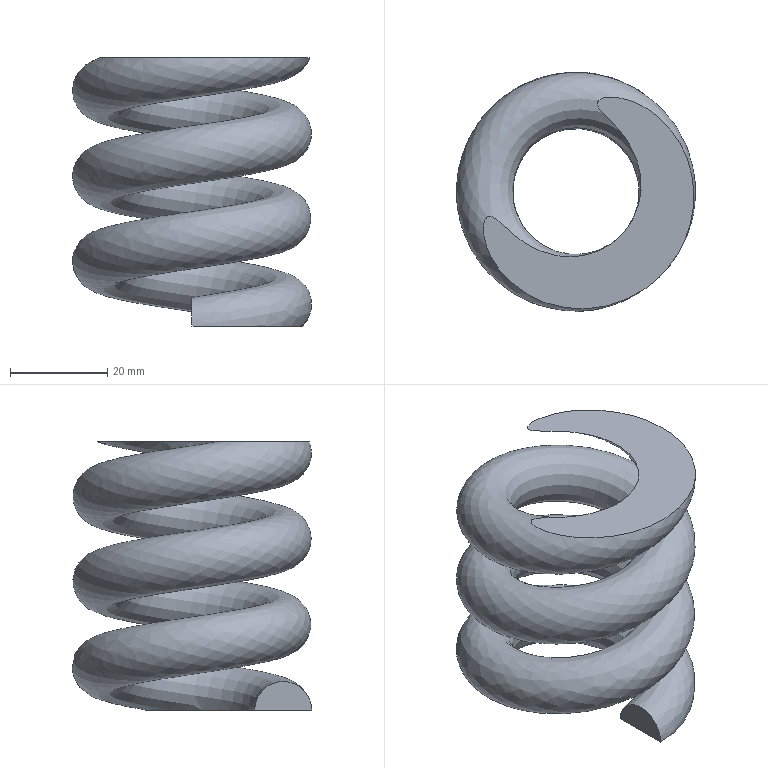Part | NX | features solid 2 | 1 solid | 4 faces | volume 38337 mm3 | plane 3 | spline 1
STEP:
#1=CARTESIAN_POINT('',(-1159.833,-619.642,-200.));
#2=VERTEX_POINT('',#1);
#3=CARTESIAN_POINT('',(-1159.833,-607.924,-200.));
#4=VERTEX_POINT('',#3);
#5=CARTESIAN_POINT('',(-1159.833,-613.783,-200.));
#6=DIRECTION('',(-1.,0.,0.));
#7=DIRECTION('',(0.,-1.,0.));
#8=AXIS2_PLACEMENT_3D('',#5,#6,#7);
#9=CIRCLE('',#8,5.859);
#10=EDGE_CURVE('',#2,#4,#9,.T.);
#11=ORIENTED_EDGE('',*,*,#10,.F.);
#12=CARTESIAN_POINT('',(-1159.833,-619.642,-200.));
#13=CARTESIAN_POINT('',(-1156.461,-619.642,-200.));
#14=CARTESIAN_POINT('',(-1151.454,-618.323,-200.));
#15=CARTESIAN_POINT('',(-1145.635,-614.786,-200.));
#16=CARTESIAN_POINT('',(-1141.941,-611.34,-200.));
#17=CARTESIAN_POINT('',(-1139.107,-607.051,-200.));
#18=CARTESIAN_POINT('',(-1137.419,-602.243,-200.));
#19=CARTESIAN_POINT('',(-1136.988,-598.021,-200.));
#20=CARTESIAN_POINT('',(-1137.288,-594.615,-200.));
#21=CARTESIAN_POINT('',(-1137.852,-592.138,-200.));
#22=CARTESIAN_POINT('',(-1138.795,-589.757,-200.));
#23=CARTESIAN_POINT('',(-1139.928,-587.928,-200.));
#24=CARTESIAN_POINT('',(-1141.068,-586.656,-200.));
#25=CARTESIAN_POINT('',(-1141.907,-585.972,-200.));
#26=CARTESIAN_POINT('',(-1142.679,-585.6,-200.));
#27=CARTESIAN_POINT('',(-1143.307,-585.474,-200.));
#28=CARTESIAN_POINT('',(-1143.919,-585.75,-200.));
#29=CARTESIAN_POINT('',(-1144.31,-586.53,-200.));
#30=CARTESIAN_POINT('',(-1144.432,-587.564,-200.));
#31=CARTESIAN_POINT('',(-1144.471,-588.818,-200.));
#32=CARTESIAN_POINT('',(-1144.484,-590.074,-200.));
#33=CARTESIAN_POINT('',(-1144.534,-591.747,-200.));
#34=CARTESIAN_POINT('',(-1144.72,-593.823,-200.));
#35=CARTESIAN_POINT('',(-1145.243,-596.307,-200.));
#36=CARTESIAN_POINT('',(-1146.08,-598.663,-200.));
#37=CARTESIAN_POINT('',(-1147.629,-601.639,-200.));
#38=CARTESIAN_POINT('',(-1150.333,-604.919,-200.));
#39=CARTESIAN_POINT('',(-1154.776,-607.425,-200.));
#40=CARTESIAN_POINT('',(-1158.142,-607.924,-200.));
#41=CARTESIAN_POINT('',(-1159.833,-607.924,-200.));
#42=B_SPLINE_CURVE_WITH_KNOTS('',3,(#12,#13,#14,#15,#16,#17,#18,#19,#20,#21,#22,#23,#24,#25,#26,#27,#28,#29,#30,#31,#32,#33,#34,#35,#36,#37,#38,#39,#40,#41),.UNSPECIFIED.,.F.,.F.,(4,1,1,1,1,1,1,1,1,1,1,1,1,1,1,1,1,1,1,1,1,1,1,1,1,1,1,4),(0.1116,0.1215,0.1265,0.1315,0.1365,0.1414,0.1464,0.1489,0.1514,0.1539,0.1564,0.1576,0.1589,0.1595,0.1601,0.1607,0.1614,0.1626,0.1639,0.1651,0.1664,0.1688,0.1713,0.1738,0.1763,0.1813,0.1863,0.1913),.UNSPECIFIED.);
#43=EDGE_CURVE('',#2,#4,#42,.T.);
#44=ORIENTED_EDGE('',*,*,#43,.T.);
#45=EDGE_LOOP('',(#11,#44));
#46=FACE_BOUND('',#45,.T.);
#47=CARTESIAN_POINT('',(-1176.496,-600.513,-145.));
#48=VERTEX_POINT('',#47);
#49=CARTESIAN_POINT('',(-1175.478,-601.297,-145.));
#50=CARTESIAN_POINT('',(-1176.301,-600.607,-145.));
#51=CARTESIAN_POINT('',(-1177.049,-600.187,-145.));
#52=CARTESIAN_POINT('',(-1177.712,-600.068,-145.));
#53=CARTESIAN_POINT('',(-1178.281,-600.447,-145.));
#54=CARTESIAN_POINT('',(-1178.67,-601.223,-145.));
#55=CARTESIAN_POINT('',(-1178.841,-602.282,-145.));
#56=CARTESIAN_POINT('',(-1178.808,-603.554,-145.));
#57=CARTESIAN_POINT('',(-1178.613,-604.806,-145.));
#58=CARTESIAN_POINT('',(-1178.177,-606.449,-145.));
#59=CARTESIAN_POINT('',(-1177.371,-608.377,-145.));
#60=CARTESIAN_POINT('',(-1176.039,-610.555,-145.));
#61=CARTESIAN_POINT('',(-1173.924,-613.138,-145.));
#62=CARTESIAN_POINT('',(-1170.662,-615.86,-145.));
#63=CARTESIAN_POINT('',(-1166.1,-618.088,-145.));
#64=CARTESIAN_POINT('',(-1161.184,-619.207,-145.));
#65=CARTESIAN_POINT('',(-1156.108,-619.164,-145.));
#66=CARTESIAN_POINT('',(-1149.523,-617.643,-145.));
#67=CARTESIAN_POINT('',(-1142.202,-613.198,-145.));
#68=CARTESIAN_POINT('',(-1137.495,-606.037,-145.));
#69=CARTESIAN_POINT('',(-1135.74,-599.515,-145.));
#70=CARTESIAN_POINT('',(-1135.504,-594.455,-145.));
#71=CARTESIAN_POINT('',(-1136.411,-589.51,-145.));
#72=CARTESIAN_POINT('',(-1138.445,-584.849,-145.));
#73=CARTESIAN_POINT('',(-1140.982,-581.484,-145.));
#74=CARTESIAN_POINT('',(-1143.469,-579.222,-145.));
#75=CARTESIAN_POINT('',(-1145.511,-577.795,-145.));
#76=CARTESIAN_POINT('',(-1147.787,-576.639,-145.));
#77=CARTESIAN_POINT('',(-1149.789,-575.994,-145.));
#78=CARTESIAN_POINT('',(-1151.467,-575.706,-145.));
#79=CARTESIAN_POINT('',(-1152.742,-575.639,-145.));
#80=CARTESIAN_POINT('',(-1153.795,-575.739,-145.));
#81=CARTESIAN_POINT('',(-1154.608,-575.989,-145.));
#82=CARTESIAN_POINT('',(-1155.181,-576.306,-145.));
#83=CARTESIAN_POINT('',(-1155.539,-576.891,-145.));
#84=CARTESIAN_POINT('',(-1155.386,-577.554,-145.));
#85=CARTESIAN_POINT('',(-1155.05,-578.094,-145.));
#86=CARTESIAN_POINT('',(-1154.509,-578.758,-145.));
#87=CARTESIAN_POINT('',(-1153.762,-579.518,-145.));
#88=CARTESIAN_POINT('',(-1152.548,-580.715,-145.));
#89=CARTESIAN_POINT('',(-1151.07,-582.261,-145.));
#90=CARTESIAN_POINT('',(-1149.001,-584.919,-145.));
#91=CARTESIAN_POINT('',(-1147.037,-588.717,-145.));
#92=CARTESIAN_POINT('',(-1146.153,-593.824,-145.));
#93=CARTESIAN_POINT('',(-1147.052,-598.911,-145.));
#94=CARTESIAN_POINT('',(-1149.587,-603.437,-145.));
#95=CARTESIAN_POINT('',(-1153.569,-606.748,-145.));
#96=CARTESIAN_POINT('',(-1158.449,-608.509,-145.));
#97=CARTESIAN_POINT('',(-1162.765,-608.529,-145.));
#98=CARTESIAN_POINT('',(-1166.065,-607.719,-145.));
#99=CARTESIAN_POINT('',(-1168.45,-606.738,-145.));
#100=CARTESIAN_POINT('',(-1170.637,-605.454,-145.));
#101=CARTESIAN_POINT('',(-1172.321,-604.169,-145.));
#102=CARTESIAN_POINT('',(-1173.605,-603.042,-145.));
#103=CARTESIAN_POINT('',(-1174.543,-602.169,-145.));
#104=CARTESIAN_POINT('',(-1175.478,-601.297,-145.));
#105=CARTESIAN_POINT('',(-1176.301,-600.607,-145.));
#106=CARTESIAN_POINT('',(-1177.049,-600.187,-145.));
#107=B_SPLINE_CURVE_WITH_KNOTS('',3,(#49,#50,#51,#52,#53,#54,#55,#56,#57,#58,#59,#60,#61,#62,#63,#64,#65,#66,#67,#68,#69,#70,#71,#72,#73,#74,#75,#76,#77,#78,#79,#80,#81,#82,#83,#84,#85,#86,#87,#88,#89,#90,#91,#92,#93,#94,#95,#96,#97,#98,#99,#100,#101,#102,#103,#104,#105,#106),.UNSPECIFIED.,.T.,.F.,(1,1,1,1,1,1,1,1,1,1,1,1,1,1,1,1,1,1,1,1,1,1,1,1,1,1,1,1,1,1,1,1,1,1,1,1,1,1,1,1,1,1,1,1,1,1,1,1,1,1,1,1,1,1,1,1,1,1,1,1,1,1),(-0.003854,-0.002569,-0.001285,0.,0.0006423,0.001285,0.001927,0.002569,0.003854,0.005139,0.006423,0.007708,0.01028,0.01285,0.01542,0.02055,0.02569,0.03083,0.03597,0.04111,0.05139,0.06166,0.0668,0.07194,0.07708,0.08222,0.08736,0.08992,0.09249,0.09506,0.09763,0.09892,0.1002,0.1015,0.1021,0.1028,0.1034,0.1041,0.1047,0.1053,0.1066,0.1079,0.1105,0.113,0.1182,0.1233,0.1285,0.1336,0.1387,0.1439,0.149,0.1516,0.1542,0.1567,0.1593,0.1606,0.1619,0.1631,0.1644,0.1651,0.1657,0.1664),.UNSPECIFIED.);
#108=EDGE_CURVE('',#48,#48,#107,.T.);
#109=ORIENTED_EDGE('',*,*,#108,.F.);
#110=EDGE_LOOP('',(#109));
#111=FACE_BOUND('',#110,.T.);
#112=CARTESIAN_POINT('',(-1159.833,-619.642,-202.072));
#113=CARTESIAN_POINT('',(-1152.8,-619.642,-201.022));
#114=CARTESIAN_POINT('',(-1141.674,-614.421,-199.349));
#115=CARTESIAN_POINT('',(-1135.098,-601.53,-197.237));
#116=CARTESIAN_POINT('',(-1134.615,-592.249,-195.881));
#117=CARTESIAN_POINT('',(-1136.656,-585.376,-194.818));
#118=CARTESIAN_POINT('',(-1140.072,-579.109,-193.76));
#119=CARTESIAN_POINT('',(-1146.949,-572.835,-192.399));
#120=CARTESIAN_POINT('',(-1157.495,-569.445,-190.788));
#121=CARTESIAN_POINT('',(-1168.422,-570.955,-189.176));
#122=CARTESIAN_POINT('',(-1177.75,-576.807,-187.572));
#123=CARTESIAN_POINT('',(-1183.583,-586.1,-185.974));
#124=CARTESIAN_POINT('',(-1185.079,-596.906,-184.381));
#125=CARTESIAN_POINT('',(-1181.753,-607.261,-182.799));
#126=CARTESIAN_POINT('',(-1174.508,-615.205,-181.227));
#127=CARTESIAN_POINT('',(-1161.467,-620.65,-179.175));
#128=CARTESIAN_POINT('',(-1143.203,-615.78,-176.599));
#129=CARTESIAN_POINT('',(-1133.842,-595.7,-173.592));
#130=CARTESIAN_POINT('',(-1142.981,-576.086,-170.655));
#131=CARTESIAN_POINT('',(-1160.033,-571.535,-168.25));
#132=CARTESIAN_POINT('',(-1171.836,-576.46,-166.393));
#133=CARTESIAN_POINT('',(-1178.201,-583.435,-165.012));
#134=CARTESIAN_POINT('',(-1181.051,-592.302,-163.658));
#135=CARTESIAN_POINT('',(-1179.8,-601.353,-162.323));
#136=CARTESIAN_POINT('',(-1175.031,-608.955,-161.016));
#137=CARTESIAN_POINT('',(-1167.571,-613.637,-159.733));
#138=CARTESIAN_POINT('',(-1159.024,-614.821,-158.473));
#139=CARTESIAN_POINT('',(-1150.959,-612.23,-157.241));
#140=CARTESIAN_POINT('',(-1145.856,-607.576,-156.231));
#141=CARTESIAN_POINT('',(-1143.291,-602.873,-155.437));
#142=CARTESIAN_POINT('',(-1141.783,-597.799,-154.652));
#143=CARTESIAN_POINT('',(-1142.124,-591.217,-153.69));
#144=CARTESIAN_POINT('',(-1146.848,-581.966,-152.174));
#145=CARTESIAN_POINT('',(-1158.976,-576.282,-150.355));
#146=CARTESIAN_POINT('',(-1170.666,-581.758,-148.602));
#147=CARTESIAN_POINT('',(-1174.966,-590.174,-147.223));
#148=CARTESIAN_POINT('',(-1175.26,-595.821,-146.398));
#149=CARTESIAN_POINT('',(-1173.986,-600.111,-145.735));
#150=CARTESIAN_POINT('',(-1171.867,-603.998,-145.078));
#151=CARTESIAN_POINT('',(-1167.875,-607.64,-144.288));
#152=CARTESIAN_POINT('',(-1161.736,-609.613,-143.35));
#153=CARTESIAN_POINT('',(-1155.458,-608.746,-142.424));
#154=CARTESIAN_POINT('',(-1150.182,-605.436,-141.517));
#155=CARTESIAN_POINT('',(-1146.924,-600.244,-140.624));
#156=CARTESIAN_POINT('',(-1146.095,-594.263,-139.742));
#157=CARTESIAN_POINT('',(-1147.916,-588.597,-138.877));
#158=CARTESIAN_POINT('',(-1151.892,-584.236,-138.014));
#159=CARTESIAN_POINT('',(-1155.646,-582.669,-137.423));
#160=CARTESIAN_POINT('',(-1157.612,-582.338,-137.126));
#161=CARTESIAN_POINT('',(-1157.698,-582.324,-137.113));
#162=CARTESIAN_POINT('',(-1159.833,-619.642,-197.928));
#163=CARTESIAN_POINT('',(-1153.407,-619.642,-196.97));
#164=CARTESIAN_POINT('',(-1142.438,-614.495,-195.32));
#165=CARTESIAN_POINT('',(-1136.013,-601.9,-193.257));
#166=CARTESIAN_POINT('',(-1135.547,-592.951,-191.949));
#167=CARTESIAN_POINT('',(-1137.506,-586.357,-190.93));
#168=CARTESIAN_POINT('',(-1140.764,-580.38,-189.92));
#169=CARTESIAN_POINT('',(-1147.245,-574.466,-188.637));
#170=CARTESIAN_POINT('',(-1157.107,-571.296,-187.131));
#171=CARTESIAN_POINT('',(-1167.228,-572.695,-185.638));
#172=CARTESIAN_POINT('',(-1175.779,-578.059,-184.168));
#173=CARTESIAN_POINT('',(-1181.074,-586.496,-182.717));
#174=CARTESIAN_POINT('',(-1182.419,-596.211,-181.284));
#175=CARTESIAN_POINT('',(-1179.458,-605.427,-179.877));
#176=CARTESIAN_POINT('',(-1173.062,-612.442,-178.488));
#177=CARTESIAN_POINT('',(-1161.607,-617.224,-176.686));
#178=CARTESIAN_POINT('',(-1145.916,-613.04,-174.473));
#179=CARTESIAN_POINT('',(-1137.949,-595.951,-171.914));
#180=CARTESIAN_POINT('',(-1145.612,-579.505,-169.451));
#181=CARTESIAN_POINT('',(-1159.634,-575.762,-167.474));
#182=CARTESIAN_POINT('',(-1169.381,-579.83,-165.94));
#183=CARTESIAN_POINT('',(-1174.564,-585.51,-164.816));
#184=CARTESIAN_POINT('',(-1176.867,-592.676,-163.721));
#185=CARTESIAN_POINT('',(-1175.859,-599.971,-162.645));
#186=CARTESIAN_POINT('',(-1172.029,-606.076,-161.596));
#187=CARTESIAN_POINT('',(-1166.052,-609.828,-160.568));
#188=CARTESIAN_POINT('',(-1159.212,-610.775,-159.559));
#189=CARTESIAN_POINT('',(-1152.771,-608.706,-158.575));
#190=CARTESIAN_POINT('',(-1148.734,-605.024,-157.776));
#191=CARTESIAN_POINT('',(-1146.65,-601.203,-157.131));
#192=CARTESIAN_POINT('',(-1145.427,-597.088,-156.495));
#193=CARTESIAN_POINT('',(-1145.698,-591.86,-155.73));
#194=CARTESIAN_POINT('',(-1149.567,-584.284,-154.489));
#195=CARTESIAN_POINT('',(-1159.375,-579.686,-153.018));
#196=CARTESIAN_POINT('',(-1168.951,-584.172,-151.582));
#197=CARTESIAN_POINT('',(-1172.594,-591.303,-150.414));
#198=CARTESIAN_POINT('',(-1172.841,-596.033,-149.722));
#199=CARTESIAN_POINT('',(-1171.743,-599.73,-149.151));
#200=CARTESIAN_POINT('',(-1169.897,-603.117,-148.579));
#201=CARTESIAN_POINT('',(-1166.452,-606.259,-147.897));
#202=CARTESIAN_POINT('',(-1161.037,-608.,-147.07));
#203=CARTESIAN_POINT('',(-1155.407,-607.222,-146.239));
#204=CARTESIAN_POINT('',(-1150.593,-604.202,-145.412));
#205=CARTESIAN_POINT('',(-1147.567,-599.381,-144.583));
#206=CARTESIAN_POINT('',(-1146.784,-593.722,-143.748));
#207=CARTESIAN_POINT('',(-1148.538,-588.261,-142.914));
#208=CARTESIAN_POINT('',(-1152.447,-583.974,-142.065));
#209=CARTESIAN_POINT('',(-1156.216,-582.4,-141.473));
#210=CARTESIAN_POINT('',(-1158.213,-582.074,-141.171));
#211=CARTESIAN_POINT('',(-1158.3,-582.061,-141.157));
#212=CARTESIAN_POINT('',(-1159.833,-618.607,-195.176));
#213=CARTESIAN_POINT('',(-1154.036,-618.607,-194.312));
#214=CARTESIAN_POINT('',(-1143.689,-613.751,-192.755));
#215=CARTESIAN_POINT('',(-1137.618,-601.848,-190.806));
#216=CARTESIAN_POINT('',(-1137.183,-593.501,-189.585));
#217=CARTESIAN_POINT('',(-1139.009,-587.352,-188.635));
#218=CARTESIAN_POINT('',(-1142.036,-581.8,-187.698));
#219=CARTESIAN_POINT('',(-1147.985,-576.372,-186.52));
#220=CARTESIAN_POINT('',(-1156.999,-573.474,-185.143));
#221=CARTESIAN_POINT('',(-1166.188,-574.745,-183.788));
#222=CARTESIAN_POINT('',(-1173.897,-579.58,-182.462));
#223=CARTESIAN_POINT('',(-1178.639,-587.135,-181.163));
#224=CARTESIAN_POINT('',(-1179.835,-595.777,-179.889));
#225=CARTESIAN_POINT('',(-1177.22,-603.918,-178.645));
#226=CARTESIAN_POINT('',(-1171.596,-610.085,-177.424));
#227=CARTESIAN_POINT('',(-1161.535,-614.286,-175.842));
#228=CARTESIAN_POINT('',(-1148.002,-610.677,-173.933));
#229=CARTESIAN_POINT('',(-1141.149,-595.978,-171.732));
#230=CARTESIAN_POINT('',(-1147.689,-581.941,-169.63));
#231=CARTESIAN_POINT('',(-1159.504,-578.788,-167.963));
#232=CARTESIAN_POINT('',(-1167.807,-582.253,-166.657));
#233=CARTESIAN_POINT('',(-1172.18,-587.045,-165.708));
#234=CARTESIAN_POINT('',(-1174.118,-593.075,-164.788));
#235=CARTESIAN_POINT('',(-1173.268,-599.225,-163.881));
#236=CARTESIAN_POINT('',(-1170.036,-604.379,-162.994));
#237=CARTESIAN_POINT('',(-1164.977,-607.553,-162.124));
#238=CARTESIAN_POINT('',(-1159.166,-608.358,-161.267));
#239=CARTESIAN_POINT('',(-1153.675,-606.594,-160.429));
#240=CARTESIAN_POINT('',(-1150.244,-603.465,-159.75));
#241=CARTESIAN_POINT('',(-1148.426,-600.132,-159.187));
#242=CARTESIAN_POINT('',(-1147.357,-596.537,-158.631));
#243=CARTESIAN_POINT('',(-1147.592,-592.022,-157.971));
#244=CARTESIAN_POINT('',(-1151.03,-585.288,-156.868));
#245=CARTESIAN_POINT('',(-1159.757,-581.198,-155.559));
#246=CARTESIAN_POINT('',(-1168.446,-585.268,-154.256));
#247=CARTESIAN_POINT('',(-1171.849,-591.928,-153.165));
#248=CARTESIAN_POINT('',(-1172.08,-596.362,-152.516));
#249=CARTESIAN_POINT('',(-1171.032,-599.89,-151.971));
#250=CARTESIAN_POINT('',(-1169.254,-603.152,-151.42));
#251=CARTESIAN_POINT('',(-1165.92,-606.193,-150.76));
#252=CARTESIAN_POINT('',(-1160.597,-607.905,-149.947));
#253=CARTESIAN_POINT('',(-1154.983,-607.129,-149.119));
#254=CARTESIAN_POINT('',(-1150.114,-604.074,-148.282));
#255=CARTESIAN_POINT('',(-1147.012,-599.131,-147.432));
#256=CARTESIAN_POINT('',(-1146.197,-593.249,-146.564));
#257=CARTESIAN_POINT('',(-1148.045,-587.497,-145.686));
#258=CARTESIAN_POINT('',(-1152.209,-582.931,-144.782));
#259=CARTESIAN_POINT('',(-1156.257,-581.241,-144.145));
#260=CARTESIAN_POINT('',(-1158.42,-580.896,-143.818));
#261=CARTESIAN_POINT('',(-1158.514,-580.882,-143.804));
#262=CARTESIAN_POINT('',(-1159.833,-615.855,-194.141));
#263=CARTESIAN_POINT('',(-1154.788,-615.855,-193.388));
#264=CARTESIAN_POINT('',(-1145.856,-611.663,-192.045));
#265=CARTESIAN_POINT('',(-1140.494,-601.152,-190.323));
#266=CARTESIAN_POINT('',(-1140.117,-593.898,-189.263));
#267=CARTESIAN_POINT('',(-1141.717,-588.51,-188.43));
#268=CARTESIAN_POINT('',(-1144.368,-583.647,-187.609));
#269=CARTESIAN_POINT('',(-1149.5,-578.964,-186.592));
#270=CARTESIAN_POINT('',(-1157.297,-576.458,-185.402));
#271=CARTESIAN_POINT('',(-1165.237,-577.555,-184.231));
#272=CARTESIAN_POINT('',(-1171.885,-581.726,-183.088));
#273=CARTESIAN_POINT('',(-1175.97,-588.234,-181.968));
#274=CARTESIAN_POINT('',(-1177.,-595.678,-180.87));
#275=CARTESIAN_POINT('',(-1174.749,-602.686,-179.8));
#276=CARTESIAN_POINT('',(-1169.894,-608.01,-178.746));
#277=CARTESIAN_POINT('',(-1161.132,-611.669,-177.368));
#278=CARTESIAN_POINT('',(-1149.436,-608.55,-175.718));
#279=CARTESIAN_POINT('',(-1143.431,-595.67,-173.789));
#280=CARTESIAN_POINT('',(-1149.225,-583.235,-171.928));
#281=CARTESIAN_POINT('',(-1159.763,-580.422,-170.441));
#282=CARTESIAN_POINT('',(-1167.343,-583.585,-169.249));
#283=CARTESIAN_POINT('',(-1171.356,-587.984,-168.378));
#284=CARTESIAN_POINT('',(-1173.152,-593.57,-167.525));
#285=CARTESIAN_POINT('',(-1172.355,-599.336,-166.674));
#286=CARTESIAN_POINT('',(-1169.286,-604.229,-165.833));
#287=CARTESIAN_POINT('',(-1164.422,-607.281,-164.997));
#288=CARTESIAN_POINT('',(-1158.757,-608.066,-164.161));
#289=CARTESIAN_POINT('',(-1153.331,-606.323,-163.333));
#290=CARTESIAN_POINT('',(-1149.894,-603.188,-162.652));
#291=CARTESIAN_POINT('',(-1148.056,-599.819,-162.083));
#292=CARTESIAN_POINT('',(-1146.966,-596.15,-161.516));
#293=CARTESIAN_POINT('',(-1147.208,-591.477,-160.833));
#294=CARTESIAN_POINT('',(-1150.799,-584.446,-159.681));
#295=CARTESIAN_POINT('',(-1160.164,-580.056,-158.276));
#296=CARTESIAN_POINT('',(-1169.701,-584.524,-156.846));
#297=CARTESIAN_POINT('',(-1173.459,-591.879,-155.641));
#298=CARTESIAN_POINT('',(-1173.722,-596.917,-154.904));
#299=CARTESIAN_POINT('',(-1172.541,-600.891,-154.29));
#300=CARTESIAN_POINT('',(-1170.53,-604.58,-153.667));
#301=CARTESIAN_POINT('',(-1166.662,-608.11,-152.901));
#302=CARTESIAN_POINT('',(-1160.486,-610.095,-151.958));
#303=CARTESIAN_POINT('',(-1153.937,-609.189,-150.992));
#304=CARTESIAN_POINT('',(-1148.22,-605.604,-150.009));
#305=CARTESIAN_POINT('',(-1144.561,-599.773,-149.006));
#306=CARTESIAN_POINT('',(-1143.597,-592.81,-147.98));
#307=CARTESIAN_POINT('',(-1145.792,-585.976,-146.936));
#308=CARTESIAN_POINT('',(-1150.735,-580.557,-145.863));
#309=CARTESIAN_POINT('',(-1155.5,-578.567,-145.113));
#310=CARTESIAN_POINT('',(-1158.06,-578.164,-144.726));
#311=CARTESIAN_POINT('',(-1158.173,-578.148,-144.71));
#312=CARTESIAN_POINT('',(-1159.833,-611.711,-194.141));
#313=CARTESIAN_POINT('',(-1155.693,-611.711,-193.523));
#314=CARTESIAN_POINT('',(-1148.831,-608.491,-192.491));
#315=CARTESIAN_POINT('',(-1144.481,-599.964,-191.094));
#316=CARTESIAN_POINT('',(-1144.183,-594.232,-190.256));
#317=CARTESIAN_POINT('',(-1145.474,-589.886,-189.585));
#318=CARTESIAN_POINT('',(-1147.62,-585.948,-188.92));
#319=CARTESIAN_POINT('',(-1151.67,-582.253,-188.118));
#320=CARTESIAN_POINT('',(-1157.893,-580.253,-187.167));
#321=CARTESIAN_POINT('',(-1164.253,-581.132,-186.229));
#322=CARTESIAN_POINT('',(-1169.597,-584.484,-185.311));
#323=CARTESIAN_POINT('',(-1172.895,-589.74,-184.407));
#324=CARTESIAN_POINT('',(-1173.733,-595.791,-183.514));
#325=CARTESIAN_POINT('',(-1171.893,-601.521,-182.639));
#326=CARTESIAN_POINT('',(-1167.875,-605.926,-181.767));
#327=CARTESIAN_POINT('',(-1160.471,-609.018,-180.603));
#328=CARTESIAN_POINT('',(-1150.573,-606.378,-179.206));
#329=CARTESIAN_POINT('',(-1145.32,-595.111,-177.519));
#330=CARTESIAN_POINT('',(-1150.545,-583.896,-175.84));
#331=CARTESIAN_POINT('',(-1160.304,-581.291,-174.463));
#332=CARTESIAN_POINT('',(-1167.567,-584.322,-173.321));
#333=CARTESIAN_POINT('',(-1171.484,-588.615,-172.471));
#334=CARTESIAN_POINT('',(-1173.271,-594.174,-171.622));
#335=CARTESIAN_POINT('',(-1172.463,-600.024,-170.759));
#336=CARTESIAN_POINT('',(-1169.287,-605.087,-169.889));
#337=CARTESIAN_POINT('',(-1164.158,-608.306,-169.007));
#338=CARTESIAN_POINT('',(-1158.071,-609.149,-168.109));
#339=CARTESIAN_POINT('',(-1152.132,-607.241,-167.202));
#340=CARTESIAN_POINT('',(-1148.285,-603.732,-166.44));
#341=CARTESIAN_POINT('',(-1146.235,-599.975,-165.806));
#342=CARTESIAN_POINT('',(-1145.005,-595.835,-165.166));
#343=CARTESIAN_POINT('',(-1145.286,-590.414,-164.373));
#344=CARTESIAN_POINT('',(-1149.427,-582.305,-163.045));
#345=CARTESIAN_POINT('',(-1160.627,-577.056,-161.365));
#346=CARTESIAN_POINT('',(-1172.236,-582.494,-159.624));
#347=CARTESIAN_POINT('',(-1176.776,-591.379,-158.168));
#348=CARTESIAN_POINT('',(-1177.104,-597.671,-157.248));
#349=CARTESIAN_POINT('',(-1175.657,-602.542,-156.495));
#350=CARTESIAN_POINT('',(-1173.194,-607.061,-155.732));
#351=CARTESIAN_POINT('',(-1168.313,-611.514,-154.766));
#352=CARTESIAN_POINT('',(-1160.582,-613.999,-153.585));
#353=CARTESIAN_POINT('',(-1152.38,-612.865,-152.376));
#354=CARTESIAN_POINT('',(-1145.214,-608.371,-151.143));
#355=CARTESIAN_POINT('',(-1140.629,-601.064,-149.887));
#356=CARTESIAN_POINT('',(-1139.423,-592.355,-148.602));
#357=CARTESIAN_POINT('',(-1142.166,-583.813,-147.298));
#358=CARTESIAN_POINT('',(-1148.306,-577.081,-145.965));
#359=CARTESIAN_POINT('',(-1154.146,-574.643,-145.047));
#360=CARTESIAN_POINT('',(-1157.294,-574.152,-144.571));
#361=CARTESIAN_POINT('',(-1157.431,-574.132,-144.55));
#362=CARTESIAN_POINT('',(-1159.833,-608.959,-195.176));
#363=CARTESIAN_POINT('',(-1156.142,-608.959,-194.626));
#364=CARTESIAN_POINT('',(-1150.616,-606.366,-193.795));
#365=CARTESIAN_POINT('',(-1146.901,-599.083,-192.602));
#366=CARTESIAN_POINT('',(-1146.651,-594.278,-191.899));
#367=CARTESIAN_POINT('',(-1147.757,-590.554,-191.324));
#368=CARTESIAN_POINT('',(-1149.607,-587.16,-190.751));
#369=CARTESIAN_POINT('',(-1153.037,-584.03,-190.071));
#370=CARTESIAN_POINT('',(-1158.385,-582.311,-189.255));
#371=CARTESIAN_POINT('',(-1163.898,-583.073,-188.442));
#372=CARTESIAN_POINT('',(-1168.57,-586.003,-187.638));
#373=CARTESIAN_POINT('',(-1171.481,-590.642,-186.841));
#374=CARTESIAN_POINT('',(-1172.228,-596.04,-186.045));
#375=CARTESIAN_POINT('',(-1170.569,-601.205,-185.256));
#376=CARTESIAN_POINT('',(-1166.896,-605.233,-184.458));
#377=CARTESIAN_POINT('',(-1159.997,-608.113,-183.373));
#378=CARTESIAN_POINT('',(-1150.65,-605.621,-182.055));
#379=CARTESIAN_POINT('',(-1145.548,-594.677,-180.416));
#380=CARTESIAN_POINT('',(-1150.765,-583.48,-178.739));
#381=CARTESIAN_POINT('',(-1160.763,-580.812,-177.329));
#382=CARTESIAN_POINT('',(-1168.33,-583.969,-176.139));
#383=CARTESIAN_POINT('',(-1172.479,-588.516,-175.239));
#384=CARTESIAN_POINT('',(-1174.397,-594.482,-174.328));
#385=CARTESIAN_POINT('',(-1173.52,-600.826,-173.392));
#386=CARTESIAN_POINT('',(-1170.038,-606.376,-172.438));
#387=CARTESIAN_POINT('',(-1164.362,-609.938,-171.462));
#388=CARTESIAN_POINT('',(-1157.568,-610.879,-170.459));
#389=CARTESIAN_POINT('',(-1150.882,-608.732,-169.439));
#390=CARTESIAN_POINT('',(-1146.496,-604.732,-168.57));
#391=CARTESIAN_POINT('',(-1144.186,-600.496,-167.855));
#392=CARTESIAN_POINT('',(-1142.791,-595.804,-167.13));
#393=CARTESIAN_POINT('',(-1143.116,-589.548,-166.215));
#394=CARTESIAN_POINT('',(-1147.836,-580.304,-164.701));
#395=CARTESIAN_POINT('',(-1160.834,-574.211,-162.751));
#396=CARTESIAN_POINT('',(-1174.349,-580.543,-160.724));
#397=CARTESIAN_POINT('',(-1179.572,-590.765,-159.049));
#398=CARTESIAN_POINT('',(-1179.955,-598.119,-157.974));
#399=CARTESIAN_POINT('',(-1178.288,-603.734,-157.106));
#400=CARTESIAN_POINT('',(-1175.456,-608.929,-156.229));
#401=CARTESIAN_POINT('',(-1169.766,-614.12,-155.102));
#402=CARTESIAN_POINT('',(-1160.82,-616.996,-153.736));
#403=CARTESIAN_POINT('',(-1151.359,-615.688,-152.341));
#404=CARTESIAN_POINT('',(-1143.115,-610.517,-150.923));
#405=CARTESIAN_POINT('',(-1137.856,-602.137,-149.482));
#406=CARTESIAN_POINT('',(-1136.478,-592.187,-148.015));
#407=CARTESIAN_POINT('',(-1139.603,-582.461,-146.529));
#408=CARTESIAN_POINT('',(-1146.554,-574.838,-145.02));
#409=CARTESIAN_POINT('',(-1153.104,-572.103,-143.99));
#410=CARTESIAN_POINT('',(-1156.634,-571.552,-143.457));
#411=CARTESIAN_POINT('',(-1156.789,-571.53,-143.433));
#412=CARTESIAN_POINT('',(-1159.833,-607.924,-197.928));
#413=CARTESIAN_POINT('',(-1155.965,-607.924,-197.351));
#414=CARTESIAN_POINT('',(-1150.852,-605.524,-196.582));
#415=CARTESIAN_POINT('',(-1147.29,-598.54,-195.438));
#416=CARTESIAN_POINT('',(-1147.048,-593.896,-194.759));
#417=CARTESIAN_POINT('',(-1148.132,-590.246,-194.195));
#418=CARTESIAN_POINT('',(-1149.961,-586.891,-193.629));
#419=CARTESIAN_POINT('',(-1153.382,-583.769,-192.951));
#420=CARTESIAN_POINT('',(-1158.791,-582.03,-192.125));
#421=CARTESIAN_POINT('',(-1164.446,-582.812,-191.291));
#422=CARTESIAN_POINT('',(-1169.307,-585.861,-190.455));
#423=CARTESIAN_POINT('',(-1172.378,-590.755,-189.614));
#424=CARTESIAN_POINT('',(-1173.178,-596.53,-188.762));
#425=CARTESIAN_POINT('',(-1171.379,-602.132,-187.907));
#426=CARTESIAN_POINT('',(-1167.352,-606.547,-187.033));
#427=CARTESIAN_POINT('',(-1159.739,-609.726,-185.835));
#428=CARTESIAN_POINT('',(-1149.132,-606.898,-184.339));
#429=CARTESIAN_POINT('',(-1143.292,-594.371,-182.463));
#430=CARTESIAN_POINT('',(-1149.347,-581.375,-180.517));
#431=CARTESIAN_POINT('',(-1161.164,-578.221,-178.85));
#432=CARTESIAN_POINT('',(-1170.016,-581.915,-177.458));
#433=CARTESIAN_POINT('',(-1174.926,-587.297,-176.392));
#434=CARTESIAN_POINT('',(-1177.205,-594.385,-175.31));
#435=CARTESIAN_POINT('',(-1176.164,-601.916,-174.199));
#436=CARTESIAN_POINT('',(-1172.032,-608.503,-173.067));
#437=CARTESIAN_POINT('',(-1165.305,-612.725,-171.91));
#438=CARTESIAN_POINT('',(-1157.271,-613.837,-170.725));
#439=CARTESIAN_POINT('',(-1149.379,-611.302,-169.52));
#440=CARTESIAN_POINT('',(-1144.182,-606.563,-168.491));
#441=CARTESIAN_POINT('',(-1141.5,-601.645,-167.66));
#442=CARTESIAN_POINT('',(-1139.88,-596.197,-166.818));
#443=CARTESIAN_POINT('',(-1140.262,-588.855,-165.745));
#444=CARTESIAN_POINT('',(-1145.687,-578.23,-164.004));
#445=CARTESIAN_POINT('',(-1160.685,-571.2,-161.755));
#446=CARTESIAN_POINT('',(-1176.122,-578.432,-159.439));
#447=CARTESIAN_POINT('',(-1181.976,-589.89,-157.562));
#448=CARTESIAN_POINT('',(-1182.408,-598.166,-156.352));
#449=CARTESIAN_POINT('',(-1180.556,-604.4,-155.389));
#450=CARTESIAN_POINT('',(-1177.43,-610.135,-154.42));
#451=CARTESIAN_POINT('',(-1171.124,-615.888,-153.171));
#452=CARTESIAN_POINT('',(-1161.308,-619.044,-151.672));
#453=CARTESIAN_POINT('',(-1151.004,-617.619,-150.153));
#454=CARTESIAN_POINT('',(-1142.091,-612.028,-148.62));
#455=CARTESIAN_POINT('',(-1136.446,-603.033,-147.073));
#456=CARTESIAN_POINT('',(-1134.978,-592.433,-145.51));
#457=CARTESIAN_POINT('',(-1138.283,-582.143,-143.938));
#458=CARTESIAN_POINT('',(-1145.579,-574.143,-142.355));
#459=CARTESIAN_POINT('',(-1152.387,-571.3,-141.284));
#460=CARTESIAN_POINT('',(-1156.043,-570.724,-140.731));
#461=CARTESIAN_POINT('',(-1156.203,-570.701,-140.707));
#462=CARTESIAN_POINT('',(-1159.833,-607.924,-202.072));
#463=CARTESIAN_POINT('',(-1155.358,-607.924,-201.404));
#464=CARTESIAN_POINT('',(-1150.088,-605.45,-200.611));
#465=CARTESIAN_POINT('',(-1146.374,-598.17,-199.419));
#466=CARTESIAN_POINT('',(-1146.115,-593.194,-198.691));
#467=CARTESIAN_POINT('',(-1147.282,-589.265,-198.084));
#468=CARTESIAN_POINT('',(-1149.27,-585.62,-197.469));
#469=CARTESIAN_POINT('',(-1153.086,-582.138,-196.713));
#470=CARTESIAN_POINT('',(-1159.179,-580.179,-195.782));
#471=CARTESIAN_POINT('',(-1165.64,-581.072,-194.83));
#472=CARTESIAN_POINT('',(-1171.278,-584.609,-193.86));
#473=CARTESIAN_POINT('',(-1174.887,-590.359,-192.871));
#474=CARTESIAN_POINT('',(-1175.838,-597.226,-191.859));
#475=CARTESIAN_POINT('',(-1173.673,-603.965,-190.829));
#476=CARTESIAN_POINT('',(-1168.798,-609.311,-189.771));
#477=CARTESIAN_POINT('',(-1159.599,-613.152,-188.324));
#478=CARTESIAN_POINT('',(-1146.419,-609.637,-186.465));
#479=CARTESIAN_POINT('',(-1139.185,-594.12,-184.141));
#480=CARTESIAN_POINT('',(-1146.716,-577.956,-181.721));
#481=CARTESIAN_POINT('',(-1161.563,-573.993,-179.627));
#482=CARTESIAN_POINT('',(-1172.471,-578.545,-177.911));
#483=CARTESIAN_POINT('',(-1178.563,-585.222,-176.589));
#484=CARTESIAN_POINT('',(-1181.389,-594.011,-175.247));
#485=CARTESIAN_POINT('',(-1180.105,-603.298,-173.877));
#486=CARTESIAN_POINT('',(-1175.034,-611.382,-172.487));
#487=CARTESIAN_POINT('',(-1166.824,-616.534,-171.075));
#488=CARTESIAN_POINT('',(-1157.083,-617.883,-169.638));
#489=CARTESIAN_POINT('',(-1147.567,-614.827,-168.185));
#490=CARTESIAN_POINT('',(-1141.304,-609.115,-166.946));
#491=CARTESIAN_POINT('',(-1138.141,-603.316,-165.966));
#492=CARTESIAN_POINT('',(-1136.236,-596.908,-164.976));
#493=CARTESIAN_POINT('',(-1136.688,-588.212,-163.704));
#494=CARTESIAN_POINT('',(-1142.969,-575.912,-161.689));
#495=CARTESIAN_POINT('',(-1160.285,-567.795,-159.092));
#496=CARTESIAN_POINT('',(-1177.837,-576.018,-156.46));
#497=CARTESIAN_POINT('',(-1184.347,-588.76,-154.372));
#498=CARTESIAN_POINT('',(-1184.827,-597.954,-153.027));
#499=CARTESIAN_POINT('',(-1182.799,-604.781,-151.973));
#500=CARTESIAN_POINT('',(-1179.4,-611.016,-150.919));
#501=CARTESIAN_POINT('',(-1172.547,-617.269,-149.562));
#502=CARTESIAN_POINT('',(-1162.007,-620.657,-147.953));
#503=CARTESIAN_POINT('',(-1151.056,-619.143,-146.338));
#504=CARTESIAN_POINT('',(-1141.68,-613.262,-144.726));
#505=CARTESIAN_POINT('',(-1135.802,-603.896,-143.115));
#506=CARTESIAN_POINT('',(-1134.289,-592.974,-141.504));
#507=CARTESIAN_POINT('',(-1137.661,-582.479,-139.901));
#508=CARTESIAN_POINT('',(-1145.024,-574.405,-138.303));
#509=CARTESIAN_POINT('',(-1151.817,-571.569,-137.234));
#510=CARTESIAN_POINT('',(-1155.443,-570.988,-136.686));
#511=CARTESIAN_POINT('',(-1155.601,-570.964,-136.662));
#512=CARTESIAN_POINT('',(-1159.833,-608.959,-204.824));
#513=CARTESIAN_POINT('',(-1154.729,-608.959,-204.062));
#514=CARTESIAN_POINT('',(-1148.837,-606.194,-203.176));
#515=CARTESIAN_POINT('',(-1144.77,-598.222,-201.87));
#516=CARTESIAN_POINT('',(-1144.479,-592.644,-201.055));
#517=CARTESIAN_POINT('',(-1145.779,-588.27,-200.379));
#518=CARTESIAN_POINT('',(-1147.997,-584.2,-199.691));
#519=CARTESIAN_POINT('',(-1152.346,-580.232,-198.83));
#520=CARTESIAN_POINT('',(-1159.287,-578.001,-197.77));
#521=CARTESIAN_POINT('',(-1166.679,-579.023,-196.68));
#522=CARTESIAN_POINT('',(-1173.16,-583.088,-195.566));
#523=CARTESIAN_POINT('',(-1177.322,-589.72,-194.425));
#524=CARTESIAN_POINT('',(-1178.422,-597.659,-193.254));
#525=CARTESIAN_POINT('',(-1175.911,-605.474,-192.061));
#526=CARTESIAN_POINT('',(-1170.263,-611.668,-190.835));
#527=CARTESIAN_POINT('',(-1159.671,-616.09,-189.169));
#528=CARTESIAN_POINT('',(-1144.333,-612.,-187.005));
#529=CARTESIAN_POINT('',(-1135.985,-594.093,-184.324));
#530=CARTESIAN_POINT('',(-1144.639,-575.52,-181.543));
#531=CARTESIAN_POINT('',(-1161.694,-570.968,-179.137));
#532=CARTESIAN_POINT('',(-1174.045,-576.122,-177.194));
#533=CARTESIAN_POINT('',(-1180.947,-583.687,-175.696));
#534=CARTESIAN_POINT('',(-1184.138,-593.612,-174.18));
#535=CARTESIAN_POINT('',(-1182.696,-604.044,-172.642));
#536=CARTESIAN_POINT('',(-1177.028,-613.08,-171.088));
#537=CARTESIAN_POINT('',(-1167.899,-618.809,-169.518));
#538=CARTESIAN_POINT('',(-1157.129,-620.3,-167.93));
#539=CARTESIAN_POINT('',(-1146.664,-616.938,-166.332));
#540=CARTESIAN_POINT('',(-1139.795,-610.674,-164.972));
#541=CARTESIAN_POINT('',(-1136.365,-604.386,-163.91));
#542=CARTESIAN_POINT('',(-1134.306,-597.459,-162.839));
#543=CARTESIAN_POINT('',(-1134.794,-588.05,-161.464));
#544=CARTESIAN_POINT('',(-1141.506,-574.908,-159.311));
#545=CARTESIAN_POINT('',(-1159.904,-566.284,-156.551));
#546=CARTESIAN_POINT('',(-1178.342,-574.922,-153.786));
#547=CARTESIAN_POINT('',(-1185.093,-588.135,-151.621));
#548=CARTESIAN_POINT('',(-1185.588,-597.625,-150.233));
#549=CARTESIAN_POINT('',(-1183.51,-604.621,-149.152));
#550=CARTESIAN_POINT('',(-1180.043,-610.981,-148.078));
#551=CARTESIAN_POINT('',(-1173.079,-617.335,-146.699));
#552=CARTESIAN_POINT('',(-1162.447,-620.753,-145.075));
#553=CARTESIAN_POINT('',(-1151.479,-619.236,-143.458));
#554=CARTESIAN_POINT('',(-1142.159,-613.39,-141.855));
#555=CARTESIAN_POINT('',(-1136.357,-604.146,-140.266));
#556=CARTESIAN_POINT('',(-1134.876,-593.447,-138.688));
#557=CARTESIAN_POINT('',(-1138.154,-583.243,-137.129));
#558=CARTESIAN_POINT('',(-1145.262,-575.448,-135.586));
#559=CARTESIAN_POINT('',(-1151.777,-572.728,-134.562));
#560=CARTESIAN_POINT('',(-1155.235,-572.166,-134.038));
#561=CARTESIAN_POINT('',(-1155.387,-572.143,-134.016));
#562=CARTESIAN_POINT('',(-1159.833,-611.711,-205.859));
#563=CARTESIAN_POINT('',(-1153.976,-611.711,-204.986));
#564=CARTESIAN_POINT('',(-1146.67,-608.282,-203.887));
#565=CARTESIAN_POINT('',(-1141.893,-598.918,-202.353));
#566=CARTESIAN_POINT('',(-1141.546,-592.247,-201.378));
#567=CARTESIAN_POINT('',(-1143.071,-587.112,-200.584));
#568=CARTESIAN_POINT('',(-1145.665,-582.353,-199.78));
#569=CARTESIAN_POINT('',(-1150.831,-577.64,-198.757));
#570=CARTESIAN_POINT('',(-1158.989,-575.017,-197.512));
#571=CARTESIAN_POINT('',(-1167.631,-576.212,-196.237));
#572=CARTESIAN_POINT('',(-1175.172,-580.942,-194.94));
#573=CARTESIAN_POINT('',(-1179.991,-588.621,-193.62));
#574=CARTESIAN_POINT('',(-1181.257,-597.758,-192.272));
#575=CARTESIAN_POINT('',(-1178.382,-606.706,-190.906));
#576=CARTESIAN_POINT('',(-1171.965,-613.743,-189.513));
#577=CARTESIAN_POINT('',(-1160.075,-618.708,-187.642));
#578=CARTESIAN_POINT('',(-1142.9,-614.128,-185.22));
#579=CARTESIAN_POINT('',(-1133.703,-594.401,-182.266));
#580=CARTESIAN_POINT('',(-1143.103,-574.226,-179.245));
#581=CARTESIAN_POINT('',(-1161.434,-569.333,-176.659));
#582=CARTESIAN_POINT('',(-1174.509,-574.79,-174.603));
#583=CARTESIAN_POINT('',(-1181.771,-582.748,-173.027));
#584=CARTESIAN_POINT('',(-1185.104,-593.117,-171.443));
#585=CARTESIAN_POINT('',(-1183.609,-603.933,-169.848));
#586=CARTESIAN_POINT('',(-1177.778,-613.229,-168.25));
#587=CARTESIAN_POINT('',(-1168.454,-619.081,-166.646));
#588=CARTESIAN_POINT('',(-1157.538,-620.592,-165.036));
#589=CARTESIAN_POINT('',(-1147.007,-617.21,-163.428));
#590=CARTESIAN_POINT('',(-1140.144,-610.951,-162.07));
#591=CARTESIAN_POINT('',(-1136.735,-604.7,-161.014));
#592=CARTESIAN_POINT('',(-1134.697,-597.846,-159.954));
#593=CARTESIAN_POINT('',(-1135.178,-588.595,-158.602));
#594=CARTESIAN_POINT('',(-1141.737,-575.75,-156.498));
#595=CARTESIAN_POINT('',(-1159.496,-567.426,-153.834));
#596=CARTESIAN_POINT('',(-1177.087,-575.666,-151.196));
#597=CARTESIAN_POINT('',(-1183.483,-588.185,-149.145));
#598=CARTESIAN_POINT('',(-1183.946,-597.071,-147.845));
#599=CARTESIAN_POINT('',(-1182.001,-603.619,-146.833));
#600=CARTESIAN_POINT('',(-1178.766,-609.553,-145.831));
#601=CARTESIAN_POINT('',(-1172.338,-615.419,-144.558));
#602=CARTESIAN_POINT('',(-1162.558,-618.563,-143.065));
#603=CARTESIAN_POINT('',(-1152.526,-617.176,-141.585));
#604=CARTESIAN_POINT('',(-1144.053,-611.861,-140.128));
#605=CARTESIAN_POINT('',(-1138.808,-603.504,-138.691));
#606=CARTESIAN_POINT('',(-1137.476,-593.886,-137.273));
#607=CARTESIAN_POINT('',(-1140.406,-584.763,-135.879));
#608=CARTESIAN_POINT('',(-1146.736,-577.823,-134.506));
#609=CARTESIAN_POINT('',(-1152.533,-575.402,-133.594));
#610=CARTESIAN_POINT('',(-1155.595,-574.897,-133.13));
#611=CARTESIAN_POINT('',(-1155.729,-574.877,-133.11));
#612=CARTESIAN_POINT('',(-1159.833,-615.855,-205.859));
#613=CARTESIAN_POINT('',(-1153.072,-615.855,-204.851));
#614=CARTESIAN_POINT('',(-1143.695,-611.454,-203.44));
#615=CARTESIAN_POINT('',(-1137.906,-600.106,-201.582));
#616=CARTESIAN_POINT('',(-1137.48,-591.913,-200.384));
#617=CARTESIAN_POINT('',(-1139.314,-585.736,-199.429));
#618=CARTESIAN_POINT('',(-1142.413,-580.052,-198.469));
#619=CARTESIAN_POINT('',(-1148.661,-574.351,-197.232));
#620=CARTESIAN_POINT('',(-1158.393,-571.222,-195.746));
#621=CARTESIAN_POINT('',(-1168.615,-572.635,-194.238));
#622=CARTESIAN_POINT('',(-1177.461,-578.184,-192.717));
#623=CARTESIAN_POINT('',(-1183.066,-587.115,-191.181));
#624=CARTESIAN_POINT('',(-1184.524,-597.645,-189.628));
#625=CARTESIAN_POINT('',(-1181.239,-607.872,-188.067));
#626=CARTESIAN_POINT('',(-1173.984,-615.827,-186.492));
#627=CARTESIAN_POINT('',(-1160.736,-621.359,-184.408));
#628=CARTESIAN_POINT('',(-1141.763,-616.299,-181.732));
#629=CARTESIAN_POINT('',(-1131.814,-594.96,-178.536));
#630=CARTESIAN_POINT('',(-1141.783,-573.565,-175.333));
#631=CARTESIAN_POINT('',(-1160.893,-568.464,-172.637));
#632=CARTESIAN_POINT('',(-1174.285,-574.053,-170.53));
#633=CARTESIAN_POINT('',(-1181.643,-582.117,-168.934));
#634=CARTESIAN_POINT('',(-1184.985,-592.513,-167.346));
#635=CARTESIAN_POINT('',(-1183.501,-603.245,-165.763));
#636=CARTESIAN_POINT('',(-1177.777,-612.371,-164.194));
#637=CARTESIAN_POINT('',(-1168.718,-618.056,-162.636));
#638=CARTESIAN_POINT('',(-1158.224,-619.51,-161.089));
#639=CARTESIAN_POINT('',(-1148.207,-616.292,-159.559));
#640=CARTESIAN_POINT('',(-1141.754,-610.407,-158.281));
#641=CARTESIAN_POINT('',(-1138.556,-604.543,-157.291));
#642=CARTESIAN_POINT('',(-1136.658,-598.161,-156.305));
#643=CARTESIAN_POINT('',(-1137.1,-589.658,-155.061));
#644=CARTESIAN_POINT('',(-1143.109,-577.891,-153.134));
#645=CARTESIAN_POINT('',(-1159.033,-570.426,-150.745));
#646=CARTESIAN_POINT('',(-1174.551,-577.696,-148.418));
#647=CARTESIAN_POINT('',(-1180.166,-588.684,-146.617));
#648=CARTESIAN_POINT('',(-1180.564,-596.316,-145.501));
#649=CARTESIAN_POINT('',(-1178.885,-601.968,-144.628));
#650=CARTESIAN_POINT('',(-1176.103,-607.072,-143.766));
#651=CARTESIAN_POINT('',(-1170.686,-612.014,-142.693));
#652=CARTESIAN_POINT('',(-1162.462,-614.658,-141.437));
#653=CARTESIAN_POINT('',(-1154.082,-613.5,-140.202));
#654=CARTESIAN_POINT('',(-1147.059,-609.094,-138.994));
#655=CARTESIAN_POINT('',(-1142.74,-602.213,-137.811));
#656=CARTESIAN_POINT('',(-1141.65,-594.341,-136.65));
#657=CARTESIAN_POINT('',(-1144.032,-586.926,-135.517));
#658=CARTESIAN_POINT('',(-1149.165,-581.298,-134.403));
#659=CARTESIAN_POINT('',(-1153.887,-579.326,-133.66));
#660=CARTESIAN_POINT('',(-1156.362,-578.91,-133.286));
#661=CARTESIAN_POINT('',(-1156.47,-578.893,-133.269));
#662=CARTESIAN_POINT('',(-1159.833,-618.607,-204.824));
#663=CARTESIAN_POINT('',(-1152.623,-618.607,-203.748));
#664=CARTESIAN_POINT('',(-1141.91,-613.579,-202.137));
#665=CARTESIAN_POINT('',(-1135.487,-600.987,-200.074));
#666=CARTESIAN_POINT('',(-1135.012,-591.867,-198.741));
#667=CARTESIAN_POINT('',(-1137.031,-585.068,-197.69));
#668=CARTESIAN_POINT('',(-1140.426,-578.84,-196.638));
#669=CARTESIAN_POINT('',(-1147.294,-572.574,-195.278));
#670=CARTESIAN_POINT('',(-1157.901,-569.164,-193.659));
#671=CARTESIAN_POINT('',(-1168.969,-570.694,-192.026));
#672=CARTESIAN_POINT('',(-1178.488,-576.664,-190.39));
#673=CARTESIAN_POINT('',(-1184.48,-586.213,-188.748));
#674=CARTESIAN_POINT('',(-1186.029,-597.396,-187.098));
#675=CARTESIAN_POINT('',(-1182.563,-608.187,-185.45));
#676=CARTESIAN_POINT('',(-1174.963,-616.52,-183.801));
#677=CARTESIAN_POINT('',(-1161.209,-622.263,-181.637));
#678=CARTESIAN_POINT('',(-1141.686,-617.057,-178.883));
#679=CARTESIAN_POINT('',(-1131.586,-595.394,-175.639));
#680=CARTESIAN_POINT('',(-1141.563,-573.981,-172.433));
#681=CARTESIAN_POINT('',(-1160.434,-568.944,-169.771));
#682=CARTESIAN_POINT('',(-1173.522,-574.405,-167.712));
#683=CARTESIAN_POINT('',(-1180.649,-582.216,-166.166));
#684=CARTESIAN_POINT('',(-1183.86,-592.205,-164.64));
#685=CARTESIAN_POINT('',(-1182.444,-602.443,-163.131));
#686=CARTESIAN_POINT('',(-1177.025,-611.082,-161.645));
#687=CARTESIAN_POINT('',(-1168.514,-616.424,-160.181));
#688=CARTESIAN_POINT('',(-1158.727,-617.779,-158.738));
#689=CARTESIAN_POINT('',(-1149.456,-614.801,-157.322));
#690=CARTESIAN_POINT('',(-1143.542,-609.407,-156.151));
#691=CARTESIAN_POINT('',(-1140.605,-604.022,-155.242));
#692=CARTESIAN_POINT('',(-1138.872,-598.192,-154.341));
#693=CARTESIAN_POINT('',(-1139.27,-590.524,-153.22));
#694=CARTESIAN_POINT('',(-1144.7,-579.892,-151.478));
#695=CARTESIAN_POINT('',(-1158.826,-573.27,-149.359));
#696=CARTESIAN_POINT('',(-1172.439,-579.647,-147.317));
#697=CARTESIAN_POINT('',(-1177.37,-589.299,-145.736));
#698=CARTESIAN_POINT('',(-1177.712,-595.868,-144.776));
#699=CARTESIAN_POINT('',(-1176.255,-600.776,-144.017));
#700=CARTESIAN_POINT('',(-1173.841,-605.203,-143.269));
#701=CARTESIAN_POINT('',(-1169.233,-609.408,-142.357));
#702=CARTESIAN_POINT('',(-1162.224,-611.661,-141.287));
#703=CARTESIAN_POINT('',(-1155.103,-610.677,-140.236));
#704=CARTESIAN_POINT('',(-1149.158,-606.948,-139.214));
#705=CARTESIAN_POINT('',(-1145.513,-601.14,-138.215));
#706=CARTESIAN_POINT('',(-1144.595,-594.509,-137.237));
#707=CARTESIAN_POINT('',(-1146.596,-588.279,-136.286));
#708=CARTESIAN_POINT('',(-1150.917,-583.541,-135.348));
#709=CARTESIAN_POINT('',(-1154.929,-581.866,-134.717));
#710=CARTESIAN_POINT('',(-1157.021,-581.51,-134.4));
#711=CARTESIAN_POINT('',(-1157.113,-581.495,-134.386));
#712=CARTESIAN_POINT('',(-1159.833,-619.642,-202.072));
#713=CARTESIAN_POINT('',(-1152.8,-619.642,-201.022));
#714=CARTESIAN_POINT('',(-1141.674,-614.421,-199.349));
#715=CARTESIAN_POINT('',(-1135.098,-601.53,-197.237));
#716=CARTESIAN_POINT('',(-1134.615,-592.249,-195.881));
#717=CARTESIAN_POINT('',(-1136.656,-585.376,-194.818));
#718=CARTESIAN_POINT('',(-1140.072,-579.109,-193.76));
#719=CARTESIAN_POINT('',(-1146.949,-572.835,-192.399));
#720=CARTESIAN_POINT('',(-1157.495,-569.445,-190.788));
#721=CARTESIAN_POINT('',(-1168.422,-570.955,-189.176));
#722=CARTESIAN_POINT('',(-1177.75,-576.807,-187.572));
#723=CARTESIAN_POINT('',(-1183.583,-586.1,-185.974));
#724=CARTESIAN_POINT('',(-1185.079,-596.906,-184.381));
#725=CARTESIAN_POINT('',(-1181.753,-607.261,-182.799));
#726=CARTESIAN_POINT('',(-1174.508,-615.205,-181.227));
#727=CARTESIAN_POINT('',(-1161.467,-620.65,-179.175));
#728=CARTESIAN_POINT('',(-1143.203,-615.78,-176.599));
#729=CARTESIAN_POINT('',(-1133.842,-595.7,-173.592));
#730=CARTESIAN_POINT('',(-1142.981,-576.086,-170.655));
#731=CARTESIAN_POINT('',(-1160.033,-571.535,-168.25));
#732=CARTESIAN_POINT('',(-1171.836,-576.46,-166.393));
#733=CARTESIAN_POINT('',(-1178.201,-583.435,-165.012));
#734=CARTESIAN_POINT('',(-1181.051,-592.302,-163.658));
#735=CARTESIAN_POINT('',(-1179.8,-601.353,-162.323));
#736=CARTESIAN_POINT('',(-1175.031,-608.955,-161.016));
#737=CARTESIAN_POINT('',(-1167.571,-613.637,-159.733));
#738=CARTESIAN_POINT('',(-1159.024,-614.821,-158.473));
#739=CARTESIAN_POINT('',(-1150.959,-612.23,-157.241));
#740=CARTESIAN_POINT('',(-1145.856,-607.576,-156.231));
#741=CARTESIAN_POINT('',(-1143.291,-602.873,-155.437));
#742=CARTESIAN_POINT('',(-1141.783,-597.799,-154.652));
#743=CARTESIAN_POINT('',(-1142.124,-591.217,-153.69));
#744=CARTESIAN_POINT('',(-1146.848,-581.966,-152.174));
#745=CARTESIAN_POINT('',(-1158.976,-576.282,-150.355));
#746=CARTESIAN_POINT('',(-1170.666,-581.758,-148.602));
#747=CARTESIAN_POINT('',(-1174.966,-590.174,-147.223));
#748=CARTESIAN_POINT('',(-1175.26,-595.821,-146.398));
#749=CARTESIAN_POINT('',(-1173.986,-600.111,-145.735));
#750=CARTESIAN_POINT('',(-1171.867,-603.998,-145.078));
#751=CARTESIAN_POINT('',(-1167.875,-607.64,-144.288));
#752=CARTESIAN_POINT('',(-1161.736,-609.613,-143.35));
#753=CARTESIAN_POINT('',(-1155.458,-608.746,-142.424));
#754=CARTESIAN_POINT('',(-1150.182,-605.436,-141.517));
#755=CARTESIAN_POINT('',(-1146.924,-600.244,-140.624));
#756=CARTESIAN_POINT('',(-1146.095,-594.263,-139.742));
#757=CARTESIAN_POINT('',(-1147.916,-588.597,-138.877));
#758=CARTESIAN_POINT('',(-1151.892,-584.236,-138.014));
#759=CARTESIAN_POINT('',(-1155.646,-582.669,-137.423));
#760=CARTESIAN_POINT('',(-1157.612,-582.338,-137.126));
#761=CARTESIAN_POINT('',(-1157.698,-582.324,-137.113));
#762=CARTESIAN_POINT('',(-1159.833,-619.642,-197.928));
#763=CARTESIAN_POINT('',(-1153.407,-619.642,-196.97));
#764=CARTESIAN_POINT('',(-1142.438,-614.495,-195.32));
#765=CARTESIAN_POINT('',(-1136.013,-601.9,-193.257));
#766=CARTESIAN_POINT('',(-1135.547,-592.951,-191.949));
#767=CARTESIAN_POINT('',(-1137.506,-586.357,-190.93));
#768=CARTESIAN_POINT('',(-1140.764,-580.38,-189.92));
#769=CARTESIAN_POINT('',(-1147.245,-574.466,-188.637));
#770=CARTESIAN_POINT('',(-1157.107,-571.296,-187.131));
#771=CARTESIAN_POINT('',(-1167.228,-572.695,-185.638));
#772=CARTESIAN_POINT('',(-1175.779,-578.059,-184.168));
#773=CARTESIAN_POINT('',(-1181.074,-586.496,-182.717));
#774=CARTESIAN_POINT('',(-1182.419,-596.211,-181.284));
#775=CARTESIAN_POINT('',(-1179.458,-605.427,-179.877));
#776=CARTESIAN_POINT('',(-1173.062,-612.442,-178.488));
#777=CARTESIAN_POINT('',(-1161.607,-617.224,-176.686));
#778=CARTESIAN_POINT('',(-1145.916,-613.04,-174.473));
#779=CARTESIAN_POINT('',(-1137.949,-595.951,-171.914));
#780=CARTESIAN_POINT('',(-1145.612,-579.505,-169.451));
#781=CARTESIAN_POINT('',(-1159.634,-575.762,-167.474));
#782=CARTESIAN_POINT('',(-1169.381,-579.83,-165.94));
#783=CARTESIAN_POINT('',(-1174.564,-585.51,-164.816));
#784=CARTESIAN_POINT('',(-1176.867,-592.676,-163.721));
#785=CARTESIAN_POINT('',(-1175.859,-599.971,-162.645));
#786=CARTESIAN_POINT('',(-1172.029,-606.076,-161.596));
#787=CARTESIAN_POINT('',(-1166.052,-609.828,-160.568));
#788=CARTESIAN_POINT('',(-1159.212,-610.775,-159.559));
#789=CARTESIAN_POINT('',(-1152.771,-608.706,-158.575));
#790=CARTESIAN_POINT('',(-1148.734,-605.024,-157.776));
#791=CARTESIAN_POINT('',(-1146.65,-601.203,-157.131));
#792=CARTESIAN_POINT('',(-1145.427,-597.088,-156.495));
#793=CARTESIAN_POINT('',(-1145.698,-591.86,-155.73));
#794=CARTESIAN_POINT('',(-1149.567,-584.284,-154.489));
#795=CARTESIAN_POINT('',(-1159.375,-579.686,-153.018));
#796=CARTESIAN_POINT('',(-1168.951,-584.172,-151.582));
#797=CARTESIAN_POINT('',(-1172.594,-591.303,-150.414));
#798=CARTESIAN_POINT('',(-1172.841,-596.033,-149.722));
#799=CARTESIAN_POINT('',(-1171.743,-599.73,-149.151));
#800=CARTESIAN_POINT('',(-1169.897,-603.117,-148.579));
#801=CARTESIAN_POINT('',(-1166.452,-606.259,-147.897));
#802=CARTESIAN_POINT('',(-1161.037,-608.,-147.07));
#803=CARTESIAN_POINT('',(-1155.407,-607.222,-146.239));
#804=CARTESIAN_POINT('',(-1150.593,-604.202,-145.412));
#805=CARTESIAN_POINT('',(-1147.567,-599.381,-144.583));
#806=CARTESIAN_POINT('',(-1146.784,-593.722,-143.748));
#807=CARTESIAN_POINT('',(-1148.538,-588.261,-142.914));
#808=CARTESIAN_POINT('',(-1152.447,-583.974,-142.065));
#809=CARTESIAN_POINT('',(-1156.216,-582.4,-141.473));
#810=CARTESIAN_POINT('',(-1158.213,-582.074,-141.171));
#811=CARTESIAN_POINT('',(-1158.3,-582.061,-141.157));
#812=(BOUNDED_SURFACE()B_SPLINE_SURFACE(4,3,((#112,#113,#114,#115,#116,#117,#118,#119,#120,#121,#122,#123,#124,#125,#126,#127,#128,#129,#130,#131,#132,#133,#134,#135,#136,#137,#138,#139,#140,#141,#142,#143,#144,#145,#146,#147,#148,#149,#150,#151,#152,#153,#154,#155,#156,#157,#158,#159,#160,#161),(#162,#163,#164,#165,#166,#167,#168,#169,#170,#171,#172,#173,#174,#175,#176,#177,#178,#179,#180,#181,#182,#183,#184,#185,#186,#187,#188,#189,#190,#191,#192,#193,#194,#195,#196,#197,#198,#199,#200,#201,#202,#203,#204,#205,#206,#207,#208,#209,#210,#211),(#212,#213,#214,#215,#216,#217,#218,#219,#220,#221,#222,#223,#224,#225,#226,#227,#228,#229,#230,#231,#232,#233,#234,#235,#236,#237,#238,#239,#240,#241,#242,#243,#244,#245,#246,#247,#248,#249,#250,#251,#252,#253,#254,#255,#256,#257,#258,#259,#260,#261),(#262,#263,#264,#265,#266,#267,#268,#269,#270,#271,#272,#273,#274,#275,#276,#277,#278,#279,#280,#281,#282,#283,#284,#285,#286,#287,#288,#289,#290,#291,#292,#293,#294,#295,#296,#297,#298,#299,#300,#301,#302,#303,#304,#305,#306,#307,#308,#309,#310,#311),(#312,#313,#314,#315,#316,#317,#318,#319,#320,#321,#322,#323,#324,#325,#326,#327,#328,#329,#330,#331,#332,#333,#334,#335,#336,#337,#338,#339,#340,#341,#342,#343,#344,#345,#346,#347,#348,#349,#350,#351,#352,#353,#354,#355,#356,#357,#358,#359,#360,#361),(#362,#363,#364,#365,#366,#367,#368,#369,#370,#371,#372,#373,#374,#375,#376,#377,#378,#379,#380,#381,#382,#383,#384,#385,#386,#387,#388,#389,#390,#391,#392,#393,#394,#395,#396,#397,#398,#399,#400,#401,#402,#403,#404,#405,#406,#407,#408,#409,#410,#411),(#412,#413,#414,#415,#416,#417,#418,#419,#420,#421,#422,#423,#424,#425,#426,#427,#428,#429,#430,#431,#432,#433,#434,#435,#436,#437,#438,#439,#440,#441,#442,#443,#444,#445,#446,#447,#448,#449,#450,#451,#452,#453,#454,#455,#456,#457,#458,#459,#460,#461),(#462,#463,#464,#465,#466,#467,#468,#469,#470,#471,#472,#473,#474,#475,#476,#477,#478,#479,#480,#481,#482,#483,#484,#485,#486,#487,#488,#489,#490,#491,#492,#493,#494,#495,#496,#497,#498,#499,#500,#501,#502,#503,#504,#505,#506,#507,#508,#509,#510,#511),(#512,#513,#514,#515,#516,#517,#518,#519,#520,#521,#522,#523,#524,#525,#526,#527,#528,#529,#530,#531,#532,#533,#534,#535,#536,#537,#538,#539,#540,#541,#542,#543,#544,#545,#546,#547,#548,#549,#550,#551,#552,#553,#554,#555,#556,#557,#558,#559,#560,#561),(#562,#563,#564,#565,#566,#567,#568,#569,#570,#571,#572,#573,#574,#575,#576,#577,#578,#579,#580,#581,#582,#583,#584,#585,#586,#587,#588,#589,#590,#591,#592,#593,#594,#595,#596,#597,#598,#599,#600,#601,#602,#603,#604,#605,#606,#607,#608,#609,#610,#611),(#612,#613,#614,#615,#616,#617,#618,#619,#620,#621,#622,#623,#624,#625,#626,#627,#628,#629,#630,#631,#632,#633,#634,#635,#636,#637,#638,#639,#640,#641,#642,#643,#644,#645,#646,#647,#648,#649,#650,#651,#652,#653,#654,#655,#656,#657,#658,#659,#660,#661),(#662,#663,#664,#665,#666,#667,#668,#669,#670,#671,#672,#673,#674,#675,#676,#677,#678,#679,#680,#681,#682,#683,#684,#685,#686,#687,#688,#689,#690,#691,#692,#693,#694,#695,#696,#697,#698,#699,#700,#701,#702,#703,#704,#705,#706,#707,#708,#709,#710,#711),(#712,#713,#714,#715,#716,#717,#718,#719,#720,#721,#722,#723,#724,#725,#726,#727,#728,#729,#730,#731,#732,#733,#734,#735,#736,#737,#738,#739,#740,#741,#742,#743,#744,#745,#746,#747,#748,#749,#750,#751,#752,#753,#754,#755,#756,#757,#758,#759,#760,#761),(#762,#763,#764,#765,#766,#767,#768,#769,#770,#771,#772,#773,#774,#775,#776,#777,#778,#779,#780,#781,#782,#783,#784,#785,#786,#787,#788,#789,#790,#791,#792,#793,#794,#795,#796,#797,#798,#799,#800,#801,#802,#803,#804,#805,#806,#807,#808,#809,#810,#811)),.UNSPECIFIED.,.T.,.F.,.F.)B_SPLINE_SURFACE_WITH_KNOTS((2,3,3,3,3,3,2),(4,1,1,1,1,1,1,1,1,1,1,1,1,1,1,1,1,1,1,1,1,1,1,1,1,1,1,1,1,1,1,1,1,1,1,1,1,1,1,1,1,1,1,1,1,1,1,4),(-0.25,0.,0.25,0.5,0.75,1.,1.25),(0.,0.01562,0.02344,0.03125,0.03516,0.03906,0.04688,0.05469,0.0625,0.07031,0.07812,0.08594,0.09375,0.1016,0.1094,0.125,0.1406,0.1562,0.1719,0.1797,0.1875,0.1953,0.2031,0.2109,0.2188,0.2266,0.2344,0.2422,0.2461,0.25,0.2578,0.2656,0.2812,0.2969,0.3047,0.3125,0.3164,0.3203,0.3281,0.3359,0.3438,0.3516,0.3594,0.3672,0.375,0.3828,0.3906,0.391),.UNSPECIFIED.)GEOMETRIC_REPRESENTATION_ITEM()RATIONAL_B_SPLINE_SURFACE(((0.5858,0.5858,0.5858,0.5858,0.5858,0.5858,0.5858,0.5858,0.5858,0.5858,0.5858,0.5858,0.5858,0.5858,0.5858,0.5858,0.5858,0.5858,0.5858,0.5858,0.5858,0.5858,0.5858,0.5858,0.5858,0.5858,0.5858,0.5858,0.5858,0.5858,0.5858,0.5858,0.5858,0.5858,0.5858,0.5858,0.5858,0.5858,0.5858,0.5858,0.5858,0.5858,0.5858,0.5858,0.5858,0.5858,0.5858,0.5858,0.5858,0.5858),(0.5858,0.5858,0.5858,0.5858,0.5858,0.5858,0.5858,0.5858,0.5858,0.5858,0.5858,0.5858,0.5858,0.5858,0.5858,0.5858,0.5858,0.5858,0.5858,0.5858,0.5858,0.5858,0.5858,0.5858,0.5858,0.5858,0.5858,0.5858,0.5858,0.5858,0.5858,0.5858,0.5858,0.5858,0.5858,0.5858,0.5858,0.5858,0.5858,0.5858,0.5858,0.5858,0.5858,0.5858,0.5858,0.5858,0.5858,0.5858,0.5858,0.5858),(0.5523,0.5523,0.5523,0.5523,0.5523,0.5523,0.5523,0.5523,0.5523,0.5523,0.5523,0.5523,0.5523,0.5523,0.5523,0.5523,0.5523,0.5523,0.5523,0.5523,0.5523,0.5523,0.5523,0.5523,0.5523,0.5523,0.5523,0.5523,0.5523,0.5523,0.5523,0.5523,0.5523,0.5523,0.5523,0.5523,0.5523,0.5523,0.5523,0.5523,0.5523,0.5523,0.5523,0.5523,0.5523,0.5523,0.5523,0.5523,0.5523,0.5523),(0.5858,0.5858,0.5858,0.5858,0.5858,0.5858,0.5858,0.5858,0.5858,0.5858,0.5858,0.5858,0.5858,0.5858,0.5858,0.5858,0.5858,0.5858,0.5858,0.5858,0.5858,0.5858,0.5858,0.5858,0.5858,0.5858,0.5858,0.5858,0.5858,0.5858,0.5858,0.5858,0.5858,0.5858,0.5858,0.5858,0.5858,0.5858,0.5858,0.5858,0.5858,0.5858,0.5858,0.5858,0.5858,0.5858,0.5858,0.5858,0.5858,0.5858),(0.5858,0.5858,0.5858,0.5858,0.5858,0.5858,0.5858,0.5858,0.5858,0.5858,0.5858,0.5858,0.5858,0.5858,0.5858,0.5858,0.5858,0.5858,0.5858,0.5858,0.5858,0.5858,0.5858,0.5858,0.5858,0.5858,0.5858,0.5858,0.5858,0.5858,0.5858,0.5858,0.5858,0.5858,0.5858,0.5858,0.5858,0.5858,0.5858,0.5858,0.5858,0.5858,0.5858,0.5858,0.5858,0.5858,0.5858,0.5858,0.5858,0.5858),(0.5523,0.5523,0.5523,0.5523,0.5523,0.5523,0.5523,0.5523,0.5523,0.5523,0.5523,0.5523,0.5523,0.5523,0.5523,0.5523,0.5523,0.5523,0.5523,0.5523,0.5523,0.5523,0.5523,0.5523,0.5523,0.5523,0.5523,0.5523,0.5523,0.5523,0.5523,0.5523,0.5523,0.5523,0.5523,0.5523,0.5523,0.5523,0.5523,0.5523,0.5523,0.5523,0.5523,0.5523,0.5523,0.5523,0.5523,0.5523,0.5523,0.5523),(0.5858,0.5858,0.5858,0.5858,0.5858,0.5858,0.5858,0.5858,0.5858,0.5858,0.5858,0.5858,0.5858,0.5858,0.5858,0.5858,0.5858,0.5858,0.5858,0.5858,0.5858,0.5858,0.5858,0.5858,0.5858,0.5858,0.5858,0.5858,0.5858,0.5858,0.5858,0.5858,0.5858,0.5858,0.5858,0.5858,0.5858,0.5858,0.5858,0.5858,0.5858,0.5858,0.5858,0.5858,0.5858,0.5858,0.5858,0.5858,0.5858,0.5858),(0.5858,0.5858,0.5858,0.5858,0.5858,0.5858,0.5858,0.5858,0.5858,0.5858,0.5858,0.5858,0.5858,0.5858,0.5858,0.5858,0.5858,0.5858,0.5858,0.5858,0.5858,0.5858,0.5858,0.5858,0.5858,0.5858,0.5858,0.5858,0.5858,0.5858,0.5858,0.5858,0.5858,0.5858,0.5858,0.5858,0.5858,0.5858,0.5858,0.5858,0.5858,0.5858,0.5858,0.5858,0.5858,0.5858,0.5858,0.5858,0.5858,0.5858),(0.5523,0.5523,0.5523,0.5523,0.5523,0.5523,0.5523,0.5523,0.5523,0.5523,0.5523,0.5523,0.5523,0.5523,0.5523,0.5523,0.5523,0.5523,0.5523,0.5523,0.5523,0.5523,0.5523,0.5523,0.5523,0.5523,0.5523,0.5523,0.5523,0.5523,0.5523,0.5523,0.5523,0.5523,0.5523,0.5523,0.5523,0.5523,0.5523,0.5523,0.5523,0.5523,0.5523,0.5523,0.5523,0.5523,0.5523,0.5523,0.5523,0.5523),(0.5858,0.5858,0.5858,0.5858,0.5858,0.5858,0.5858,0.5858,0.5858,0.5858,0.5858,0.5858,0.5858,0.5858,0.5858,0.5858,0.5858,0.5858,0.5858,0.5858,0.5858,0.5858,0.5858,0.5858,0.5858,0.5858,0.5858,0.5858,0.5858,0.5858,0.5858,0.5858,0.5858,0.5858,0.5858,0.5858,0.5858,0.5858,0.5858,0.5858,0.5858,0.5858,0.5858,0.5858,0.5858,0.5858,0.5858,0.5858,0.5858,0.5858),(0.5858,0.5858,0.5858,0.5858,0.5858,0.5858,0.5858,0.5858,0.5858,0.5858,0.5858,0.5858,0.5858,0.5858,0.5858,0.5858,0.5858,0.5858,0.5858,0.5858,0.5858,0.5858,0.5858,0.5858,0.5858,0.5858,0.5858,0.5858,0.5858,0.5858,0.5858,0.5858,0.5858,0.5858,0.5858,0.5858,0.5858,0.5858,0.5858,0.5858,0.5858,0.5858,0.5858,0.5858,0.5858,0.5858,0.5858,0.5858,0.5858,0.5858),(0.5523,0.5523,0.5523,0.5523,0.5523,0.5523,0.5523,0.5523,0.5523,0.5523,0.5523,0.5523,0.5523,0.5523,0.5523,0.5523,0.5523,0.5523,0.5523,0.5523,0.5523,0.5523,0.5523,0.5523,0.5523,0.5523,0.5523,0.5523,0.5523,0.5523,0.5523,0.5523,0.5523,0.5523,0.5523,0.5523,0.5523,0.5523,0.5523,0.5523,0.5523,0.5523,0.5523,0.5523,0.5523,0.5523,0.5523,0.5523,0.5523,0.5523),(0.5858,0.5858,0.5858,0.5858,0.5858,0.5858,0.5858,0.5858,0.5858,0.5858,0.5858,0.5858,0.5858,0.5858,0.5858,0.5858,0.5858,0.5858,0.5858,0.5858,0.5858,0.5858,0.5858,0.5858,0.5858,0.5858,0.5858,0.5858,0.5858,0.5858,0.5858,0.5858,0.5858,0.5858,0.5858,0.5858,0.5858,0.5858,0.5858,0.5858,0.5858,0.5858,0.5858,0.5858,0.5858,0.5858,0.5858,0.5858,0.5858,0.5858),(0.5858,0.5858,0.5858,0.5858,0.5858,0.5858,0.5858,0.5858,0.5858,0.5858,0.5858,0.5858,0.5858,0.5858,0.5858,0.5858,0.5858,0.5858,0.5858,0.5858,0.5858,0.5858,0.5858,0.5858,0.5858,0.5858,0.5858,0.5858,0.5858,0.5858,0.5858,0.5858,0.5858,0.5858,0.5858,0.5858,0.5858,0.5858,0.5858,0.5858,0.5858,0.5858,0.5858,0.5858,0.5858,0.5858,0.5858,0.5858,0.5858,0.5858)))REPRESENTATION_ITEM('')SURFACE());
#813=ADVANCED_FACE('',(#46,#111),#812,.F.);
#814=CARTESIAN_POINT('',(-1159.833,-613.783,-200.));
#815=DIRECTION('',(0.,1.,0.));
#816=VECTOR('',#815,1000.);
#817=LINE('',#814,#816);
#818=EDGE_CURVE('',#2,#4,#817,.T.);
#819=ORIENTED_EDGE('',*,*,#818,.F.);
#820=ORIENTED_EDGE('',*,*,#10,.T.);
#821=EDGE_LOOP('',(#819,#820));
#822=FACE_BOUND('',#821,.T.);
#823=CARTESIAN_POINT('',(-1159.833,-613.783,-200.));
#824=DIRECTION('',(-1.,0.,0.));
#825=DIRECTION('',(0.,-1.,0.));
#826=AXIS2_PLACEMENT_3D('',#823,#824,#825);
#827=PLANE('',#826);
#828=ADVANCED_FACE('',(#822),#827,.T.);
#829=ORIENTED_EDGE('',*,*,#108,.T.);
#830=EDGE_LOOP('',(#829));
#831=FACE_BOUND('',#830,.T.);
#832=CARTESIAN_POINT('',(-1159.833,-595.033,-145.));
#833=DIRECTION('',(0.,0.,1.));
#834=DIRECTION('',(0.,-1.,0.));
#835=AXIS2_PLACEMENT_3D('',#832,#833,#834);
#836=PLANE('',#835);
#837=ADVANCED_FACE('',(#831),#836,.T.);
#838=ORIENTED_EDGE('',*,*,#43,.F.);
#839=ORIENTED_EDGE('',*,*,#818,.T.);
#840=EDGE_LOOP('',(#838,#839));
#841=FACE_BOUND('',#840,.T.);
#842=CARTESIAN_POINT('',(-1159.833,-595.033,-200.));
#843=DIRECTION('',(0.,0.,1.));
#844=DIRECTION('',(0.,-1.,0.));
#845=AXIS2_PLACEMENT_3D('',#842,#843,#844);
#846=PLANE('',#845);
#847=ADVANCED_FACE('',(#841),#846,.F.);
#848=CLOSED_SHELL('',(#813,#828,#837,#847));
#849=MANIFOLD_SOLID_BREP('',#848);
#850=(LENGTH_UNIT()NAMED_UNIT(*)SI_UNIT(.MILLI.,.METRE.));
#851=UNCERTAINTY_MEASURE_WITH_UNIT(LENGTH_MEASURE(0.0508),#850,'','');
#852=(NAMED_UNIT(*)PLANE_ANGLE_UNIT()SI_UNIT($,.RADIAN.));
#853=(NAMED_UNIT(*)SI_UNIT($,.STERADIAN.)SOLID_ANGLE_UNIT());
#854=(GEOMETRIC_REPRESENTATION_CONTEXT(3)GLOBAL_UNCERTAINTY_ASSIGNED_CONTEXT((#851))GLOBAL_UNIT_ASSIGNED_CONTEXT((#850,#852,#853))REPRESENTATION_CONTEXT('',''));
#855=ADVANCED_BREP_SHAPE_REPRESENTATION('',(#849),#854);